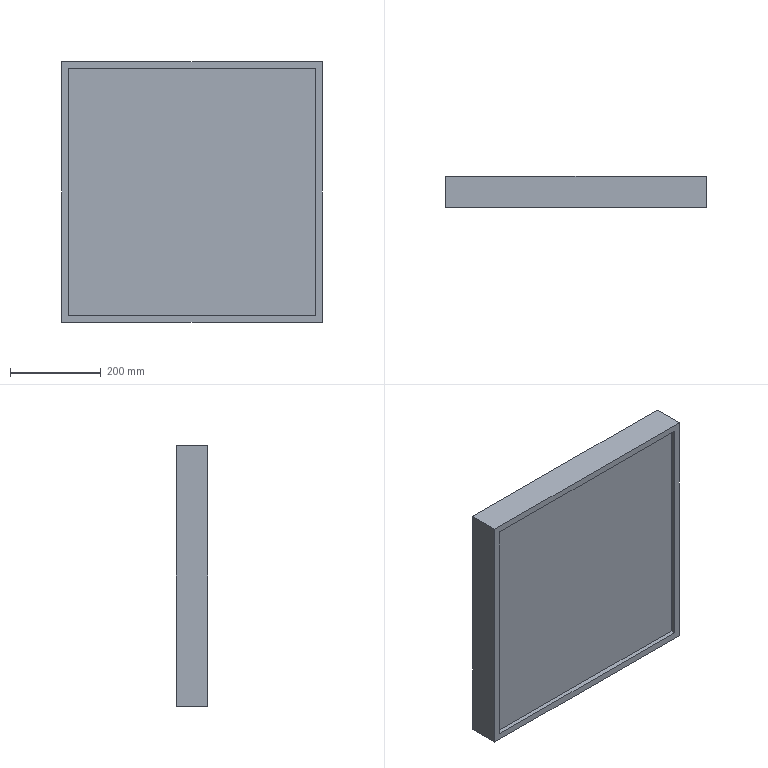Part | STEP file | FFUfilter | 1 solid | 11 faces | box 575 x 69 x 575 mm | volume 19842875 mm3 | plane 11
STEP:
#1=CARTESIAN_POINT('',(0.,0.,0.));
#2=DIRECTION('',(0.,0.,1.));
#3=DIRECTION('',(1.,0.,0.));
#4=AXIS2_PLACEMENT_3D('',#1,#2,#3);
#5=CARTESIAN_POINT('',(-287.5,0.,-287.5));
#6=VERTEX_POINT('',#5);
#7=CARTESIAN_POINT('',(-287.5,0.,287.5));
#8=VERTEX_POINT('',#7);
#9=CARTESIAN_POINT('',(-287.5,0.,-287.5));
#10=DIRECTION('',(0.,0.,1.));
#11=VECTOR('',#10,1.);
#12=LINE('',#9,#11);
#13=CARTESIAN_POINT('',(-287.5,69.,-287.5));
#14=DIRECTION('',(1.,0.,0.));
#15=DIRECTION('',(0.,0.,-1.));
#16=AXIS2_PLACEMENT_3D('',#13,#14,#15);
#17=PLANE('',#16);
#18=CARTESIAN_POINT('',(0.,-69.));
#19=DIRECTION('',(-1.,0.));
#20=VECTOR('',#19,1.);
#21=LINE('',#18,#20);
#22=(GEOMETRIC_REPRESENTATION_CONTEXT(2)PARAMETRIC_REPRESENTATION_CONTEXT()REPRESENTATION_CONTEXT('',''));
#23=DEFINITIONAL_REPRESENTATION('',(#21),#22);
#24=PCURVE('',#17,#23);
#25=CARTESIAN_POINT('',(0.,0.,0.));
#26=DIRECTION('',(0.,1.,0.));
#27=DIRECTION('',(0.,0.,1.));
#28=AXIS2_PLACEMENT_3D('',#25,#26,#27);
#29=PLANE('',#28);
#30=CARTESIAN_POINT('',(-287.5,-287.5));
#31=DIRECTION('',(1.,0.));
#32=VECTOR('',#31,1.);
#33=LINE('',#30,#32);
#34=(GEOMETRIC_REPRESENTATION_CONTEXT(2)PARAMETRIC_REPRESENTATION_CONTEXT()REPRESENTATION_CONTEXT('',''));
#35=DEFINITIONAL_REPRESENTATION('',(#33),#34);
#36=PCURVE('',#29,#35);
#37=SURFACE_CURVE('',#12,(#24,#36),.PCURVE_S1.);
#38=EDGE_CURVE('',#6,#8,#37,.T.);
#39=ORIENTED_EDGE('',*,*,#38,.T.);
#40=CARTESIAN_POINT('',(-287.5,69.,287.5));
#41=VERTEX_POINT('',#40);
#42=CARTESIAN_POINT('',(-287.5,69.,287.5));
#43=DIRECTION('',(0.,-1.,0.));
#44=VECTOR('',#43,1.);
#45=LINE('',#42,#44);
#46=CARTESIAN_POINT('',(-575.,0.));
#47=DIRECTION('',(0.,-1.));
#48=VECTOR('',#47,1.);
#49=LINE('',#46,#48);
#50=(GEOMETRIC_REPRESENTATION_CONTEXT(2)PARAMETRIC_REPRESENTATION_CONTEXT()REPRESENTATION_CONTEXT('',''));
#51=DEFINITIONAL_REPRESENTATION('',(#49),#50);
#52=PCURVE('',#17,#51);
#53=CARTESIAN_POINT('',(-287.5,69.,287.5));
#54=DIRECTION('',(0.,0.,-1.));
#55=DIRECTION('',(-1.,0.,0.));
#56=AXIS2_PLACEMENT_3D('',#53,#54,#55);
#57=PLANE('',#56);
#58=CARTESIAN_POINT('',(0.,0.));
#59=DIRECTION('',(0.,-1.));
#60=VECTOR('',#59,1.);
#61=LINE('',#58,#60);
#62=(GEOMETRIC_REPRESENTATION_CONTEXT(2)PARAMETRIC_REPRESENTATION_CONTEXT()REPRESENTATION_CONTEXT('',''));
#63=DEFINITIONAL_REPRESENTATION('',(#61),#62);
#64=PCURVE('',#57,#63);
#65=SURFACE_CURVE('',#45,(#52,#64),.PCURVE_S1.);
#66=EDGE_CURVE('',#41,#8,#65,.T.);
#67=ORIENTED_EDGE('',*,*,#66,.F.);
#68=CARTESIAN_POINT('',(-287.5,69.,-287.5));
#69=VERTEX_POINT('',#68);
#70=CARTESIAN_POINT('',(-287.5,69.,-287.5));
#71=DIRECTION('',(0.,0.,1.));
#72=VECTOR('',#71,1.);
#73=LINE('',#70,#72);
#74=CARTESIAN_POINT('',(0.,0.));
#75=DIRECTION('',(-1.,0.));
#76=VECTOR('',#75,1.);
#77=LINE('',#74,#76);
#78=(GEOMETRIC_REPRESENTATION_CONTEXT(2)PARAMETRIC_REPRESENTATION_CONTEXT()REPRESENTATION_CONTEXT('',''));
#79=DEFINITIONAL_REPRESENTATION('',(#77),#78);
#80=PCURVE('',#17,#79);
#81=CARTESIAN_POINT('',(0.,69.,0.));
#82=DIRECTION('',(0.,1.,0.));
#83=DIRECTION('',(0.,0.,1.));
#84=AXIS2_PLACEMENT_3D('',#81,#82,#83);
#85=PLANE('',#84);
#86=CARTESIAN_POINT('',(-287.5,-287.5));
#87=DIRECTION('',(1.,0.));
#88=VECTOR('',#87,1.);
#89=LINE('',#86,#88);
#90=(GEOMETRIC_REPRESENTATION_CONTEXT(2)PARAMETRIC_REPRESENTATION_CONTEXT()REPRESENTATION_CONTEXT('',''));
#91=DEFINITIONAL_REPRESENTATION('',(#89),#90);
#92=PCURVE('',#85,#91);
#93=SURFACE_CURVE('',#73,(#80,#92),.PCURVE_S1.);
#94=EDGE_CURVE('',#69,#41,#93,.T.);
#95=ORIENTED_EDGE('',*,*,#94,.F.);
#96=CARTESIAN_POINT('',(-287.5,69.,-287.5));
#97=DIRECTION('',(0.,-1.,0.));
#98=VECTOR('',#97,1.);
#99=LINE('',#96,#98);
#100=CARTESIAN_POINT('',(0.,0.));
#101=DIRECTION('',(0.,-1.));
#102=VECTOR('',#101,1.);
#103=LINE('',#100,#102);
#104=(GEOMETRIC_REPRESENTATION_CONTEXT(2)PARAMETRIC_REPRESENTATION_CONTEXT()REPRESENTATION_CONTEXT('',''));
#105=DEFINITIONAL_REPRESENTATION('',(#103),#104);
#106=PCURVE('',#17,#105);
#107=CARTESIAN_POINT('',(-287.5,69.,-287.5));
#108=DIRECTION('',(0.,0.,1.));
#109=DIRECTION('',(1.,0.,0.));
#110=AXIS2_PLACEMENT_3D('',#107,#108,#109);
#111=PLANE('',#110);
#112=CARTESIAN_POINT('',(0.,0.));
#113=DIRECTION('',(0.,-1.));
#114=VECTOR('',#113,1.);
#115=LINE('',#112,#114);
#116=(GEOMETRIC_REPRESENTATION_CONTEXT(2)PARAMETRIC_REPRESENTATION_CONTEXT()REPRESENTATION_CONTEXT('',''));
#117=DEFINITIONAL_REPRESENTATION('',(#115),#116);
#118=PCURVE('',#111,#117);
#119=SURFACE_CURVE('',#99,(#106,#118),.PCURVE_S1.);
#120=EDGE_CURVE('',#69,#6,#119,.T.);
#121=ORIENTED_EDGE('',*,*,#120,.T.);
#122=EDGE_LOOP('',(#39,#67,#95,#121));
#123=FACE_BOUND('',#122,.T.);
#124=ADVANCED_FACE('',(#123),#17,.F.);
#125=CARTESIAN_POINT('',(287.5,0.,287.5));
#126=VERTEX_POINT('',#125);
#127=CARTESIAN_POINT('',(-287.5,0.,287.5));
#128=DIRECTION('',(1.,0.,0.));
#129=VECTOR('',#128,1.);
#130=LINE('',#127,#129);
#131=CARTESIAN_POINT('',(0.,-69.));
#132=DIRECTION('',(-1.,0.));
#133=VECTOR('',#132,1.);
#134=LINE('',#131,#133);
#135=(GEOMETRIC_REPRESENTATION_CONTEXT(2)PARAMETRIC_REPRESENTATION_CONTEXT()REPRESENTATION_CONTEXT('',''));
#136=DEFINITIONAL_REPRESENTATION('',(#134),#135);
#137=PCURVE('',#57,#136);
#138=CARTESIAN_POINT('',(287.5,-287.5));
#139=DIRECTION('',(0.,1.));
#140=VECTOR('',#139,1.);
#141=LINE('',#138,#140);
#142=(GEOMETRIC_REPRESENTATION_CONTEXT(2)PARAMETRIC_REPRESENTATION_CONTEXT()REPRESENTATION_CONTEXT('',''));
#143=DEFINITIONAL_REPRESENTATION('',(#141),#142);
#144=PCURVE('',#29,#143);
#145=SURFACE_CURVE('',#130,(#137,#144),.PCURVE_S1.);
#146=EDGE_CURVE('',#8,#126,#145,.T.);
#147=ORIENTED_EDGE('',*,*,#146,.T.);
#148=CARTESIAN_POINT('',(287.5,69.,287.5));
#149=VERTEX_POINT('',#148);
#150=CARTESIAN_POINT('',(287.5,69.,287.5));
#151=DIRECTION('',(0.,-1.,0.));
#152=VECTOR('',#151,1.);
#153=LINE('',#150,#152);
#154=CARTESIAN_POINT('',(-575.,0.));
#155=DIRECTION('',(0.,-1.));
#156=VECTOR('',#155,1.);
#157=LINE('',#154,#156);
#158=(GEOMETRIC_REPRESENTATION_CONTEXT(2)PARAMETRIC_REPRESENTATION_CONTEXT()REPRESENTATION_CONTEXT('',''));
#159=DEFINITIONAL_REPRESENTATION('',(#157),#158);
#160=PCURVE('',#57,#159);
#161=CARTESIAN_POINT('',(287.5,69.,-287.5));
#162=DIRECTION('',(-1.,0.,0.));
#163=DIRECTION('',(0.,0.,1.));
#164=AXIS2_PLACEMENT_3D('',#161,#162,#163);
#165=PLANE('',#164);
#166=CARTESIAN_POINT('',(575.,0.));
#167=DIRECTION('',(0.,-1.));
#168=VECTOR('',#167,1.);
#169=LINE('',#166,#168);
#170=(GEOMETRIC_REPRESENTATION_CONTEXT(2)PARAMETRIC_REPRESENTATION_CONTEXT()REPRESENTATION_CONTEXT('',''));
#171=DEFINITIONAL_REPRESENTATION('',(#169),#170);
#172=PCURVE('',#165,#171);
#173=SURFACE_CURVE('',#153,(#160,#172),.PCURVE_S1.);
#174=EDGE_CURVE('',#149,#126,#173,.T.);
#175=ORIENTED_EDGE('',*,*,#174,.F.);
#176=CARTESIAN_POINT('',(-287.5,69.,287.5));
#177=DIRECTION('',(1.,0.,0.));
#178=VECTOR('',#177,1.);
#179=LINE('',#176,#178);
#180=CARTESIAN_POINT('',(0.,0.));
#181=DIRECTION('',(-1.,0.));
#182=VECTOR('',#181,1.);
#183=LINE('',#180,#182);
#184=(GEOMETRIC_REPRESENTATION_CONTEXT(2)PARAMETRIC_REPRESENTATION_CONTEXT()REPRESENTATION_CONTEXT('',''));
#185=DEFINITIONAL_REPRESENTATION('',(#183),#184);
#186=PCURVE('',#57,#185);
#187=CARTESIAN_POINT('',(287.5,-287.5));
#188=DIRECTION('',(0.,1.));
#189=VECTOR('',#188,1.);
#190=LINE('',#187,#189);
#191=(GEOMETRIC_REPRESENTATION_CONTEXT(2)PARAMETRIC_REPRESENTATION_CONTEXT()REPRESENTATION_CONTEXT('',''));
#192=DEFINITIONAL_REPRESENTATION('',(#190),#191);
#193=PCURVE('',#85,#192);
#194=SURFACE_CURVE('',#179,(#186,#193),.PCURVE_S1.);
#195=EDGE_CURVE('',#41,#149,#194,.T.);
#196=ORIENTED_EDGE('',*,*,#195,.F.);
#197=ORIENTED_EDGE('',*,*,#66,.T.);
#198=EDGE_LOOP('',(#147,#175,#196,#197));
#199=FACE_BOUND('',#198,.T.);
#200=ADVANCED_FACE('',(#199),#57,.F.);
#201=CARTESIAN_POINT('',(287.5,0.,-287.5));
#202=VERTEX_POINT('',#201);
#203=CARTESIAN_POINT('',(287.5,0.,-287.5));
#204=DIRECTION('',(0.,0.,-1.));
#205=VECTOR('',#204,1.);
#206=LINE('',#203,#205);
#207=CARTESIAN_POINT('',(0.,-69.));
#208=DIRECTION('',(-1.,0.));
#209=VECTOR('',#208,1.);
#210=LINE('',#207,#209);
#211=(GEOMETRIC_REPRESENTATION_CONTEXT(2)PARAMETRIC_REPRESENTATION_CONTEXT()REPRESENTATION_CONTEXT('',''));
#212=DEFINITIONAL_REPRESENTATION('',(#210),#211);
#213=PCURVE('',#165,#212);
#214=CARTESIAN_POINT('',(-287.5,287.5));
#215=DIRECTION('',(-1.,0.));
#216=VECTOR('',#215,1.);
#217=LINE('',#214,#216);
#218=(GEOMETRIC_REPRESENTATION_CONTEXT(2)PARAMETRIC_REPRESENTATION_CONTEXT()REPRESENTATION_CONTEXT('',''));
#219=DEFINITIONAL_REPRESENTATION('',(#217),#218);
#220=PCURVE('',#29,#219);
#221=SURFACE_CURVE('',#206,(#213,#220),.PCURVE_S1.);
#222=EDGE_CURVE('',#126,#202,#221,.T.);
#223=ORIENTED_EDGE('',*,*,#222,.T.);
#224=CARTESIAN_POINT('',(287.5,69.,-287.5));
#225=VERTEX_POINT('',#224);
#226=CARTESIAN_POINT('',(287.5,69.,-287.5));
#227=DIRECTION('',(0.,-1.,0.));
#228=VECTOR('',#227,1.);
#229=LINE('',#226,#228);
#230=CARTESIAN_POINT('',(0.,0.));
#231=DIRECTION('',(0.,-1.));
#232=VECTOR('',#231,1.);
#233=LINE('',#230,#232);
#234=(GEOMETRIC_REPRESENTATION_CONTEXT(2)PARAMETRIC_REPRESENTATION_CONTEXT()REPRESENTATION_CONTEXT('',''));
#235=DEFINITIONAL_REPRESENTATION('',(#233),#234);
#236=PCURVE('',#165,#235);
#237=CARTESIAN_POINT('',(575.,0.));
#238=DIRECTION('',(0.,-1.));
#239=VECTOR('',#238,1.);
#240=LINE('',#237,#239);
#241=(GEOMETRIC_REPRESENTATION_CONTEXT(2)PARAMETRIC_REPRESENTATION_CONTEXT()REPRESENTATION_CONTEXT('',''));
#242=DEFINITIONAL_REPRESENTATION('',(#240),#241);
#243=PCURVE('',#111,#242);
#244=SURFACE_CURVE('',#229,(#236,#243),.PCURVE_S1.);
#245=EDGE_CURVE('',#225,#202,#244,.T.);
#246=ORIENTED_EDGE('',*,*,#245,.F.);
#247=CARTESIAN_POINT('',(287.5,69.,-287.5));
#248=DIRECTION('',(0.,0.,-1.));
#249=VECTOR('',#248,1.);
#250=LINE('',#247,#249);
#251=CARTESIAN_POINT('',(0.,0.));
#252=DIRECTION('',(-1.,0.));
#253=VECTOR('',#252,1.);
#254=LINE('',#251,#253);
#255=(GEOMETRIC_REPRESENTATION_CONTEXT(2)PARAMETRIC_REPRESENTATION_CONTEXT()REPRESENTATION_CONTEXT('',''));
#256=DEFINITIONAL_REPRESENTATION('',(#254),#255);
#257=PCURVE('',#165,#256);
#258=CARTESIAN_POINT('',(-287.5,287.5));
#259=DIRECTION('',(-1.,0.));
#260=VECTOR('',#259,1.);
#261=LINE('',#258,#260);
#262=(GEOMETRIC_REPRESENTATION_CONTEXT(2)PARAMETRIC_REPRESENTATION_CONTEXT()REPRESENTATION_CONTEXT('',''));
#263=DEFINITIONAL_REPRESENTATION('',(#261),#262);
#264=PCURVE('',#85,#263);
#265=SURFACE_CURVE('',#250,(#257,#264),.PCURVE_S1.);
#266=EDGE_CURVE('',#149,#225,#265,.T.);
#267=ORIENTED_EDGE('',*,*,#266,.F.);
#268=ORIENTED_EDGE('',*,*,#174,.T.);
#269=EDGE_LOOP('',(#223,#246,#267,#268));
#270=FACE_BOUND('',#269,.T.);
#271=ADVANCED_FACE('',(#270),#165,.F.);
#272=CARTESIAN_POINT('',(-287.5,0.,-287.5));
#273=DIRECTION('',(-1.,0.,0.));
#274=VECTOR('',#273,1.);
#275=LINE('',#272,#274);
#276=CARTESIAN_POINT('',(0.,-69.));
#277=DIRECTION('',(-1.,0.));
#278=VECTOR('',#277,1.);
#279=LINE('',#276,#278);
#280=(GEOMETRIC_REPRESENTATION_CONTEXT(2)PARAMETRIC_REPRESENTATION_CONTEXT()REPRESENTATION_CONTEXT('',''));
#281=DEFINITIONAL_REPRESENTATION('',(#279),#280);
#282=PCURVE('',#111,#281);
#283=CARTESIAN_POINT('',(-287.5,-287.5));
#284=DIRECTION('',(0.,-1.));
#285=VECTOR('',#284,1.);
#286=LINE('',#283,#285);
#287=(GEOMETRIC_REPRESENTATION_CONTEXT(2)PARAMETRIC_REPRESENTATION_CONTEXT()REPRESENTATION_CONTEXT('',''));
#288=DEFINITIONAL_REPRESENTATION('',(#286),#287);
#289=PCURVE('',#29,#288);
#290=SURFACE_CURVE('',#275,(#282,#289),.PCURVE_S1.);
#291=EDGE_CURVE('',#202,#6,#290,.T.);
#292=ORIENTED_EDGE('',*,*,#291,.T.);
#293=ORIENTED_EDGE('',*,*,#120,.F.);
#294=CARTESIAN_POINT('',(-287.5,69.,-287.5));
#295=DIRECTION('',(-1.,0.,0.));
#296=VECTOR('',#295,1.);
#297=LINE('',#294,#296);
#298=CARTESIAN_POINT('',(0.,0.));
#299=DIRECTION('',(-1.,0.));
#300=VECTOR('',#299,1.);
#301=LINE('',#298,#300);
#302=(GEOMETRIC_REPRESENTATION_CONTEXT(2)PARAMETRIC_REPRESENTATION_CONTEXT()REPRESENTATION_CONTEXT('',''));
#303=DEFINITIONAL_REPRESENTATION('',(#301),#302);
#304=PCURVE('',#111,#303);
#305=CARTESIAN_POINT('',(-287.5,-287.5));
#306=DIRECTION('',(0.,-1.));
#307=VECTOR('',#306,1.);
#308=LINE('',#305,#307);
#309=(GEOMETRIC_REPRESENTATION_CONTEXT(2)PARAMETRIC_REPRESENTATION_CONTEXT()REPRESENTATION_CONTEXT('',''));
#310=DEFINITIONAL_REPRESENTATION('',(#308),#309);
#311=PCURVE('',#85,#310);
#312=SURFACE_CURVE('',#297,(#304,#311),.PCURVE_S1.);
#313=EDGE_CURVE('',#225,#69,#312,.T.);
#314=ORIENTED_EDGE('',*,*,#313,.F.);
#315=ORIENTED_EDGE('',*,*,#245,.T.);
#316=EDGE_LOOP('',(#292,#293,#314,#315));
#317=FACE_BOUND('',#316,.T.);
#318=ADVANCED_FACE('',(#317),#111,.F.);
#319=ORIENTED_EDGE('',*,*,#94,.T.);
#320=ORIENTED_EDGE('',*,*,#195,.T.);
#321=ORIENTED_EDGE('',*,*,#266,.T.);
#322=ORIENTED_EDGE('',*,*,#313,.T.);
#323=EDGE_LOOP('',(#319,#320,#321,#322));
#324=FACE_BOUND('',#323,.T.);
#325=ADVANCED_FACE('',(#324),#85,.T.);
#326=CARTESIAN_POINT('',(-272.5,0.,-272.5));
#327=VERTEX_POINT('',#326);
#328=CARTESIAN_POINT('',(272.5,0.,-272.5));
#329=VERTEX_POINT('',#328);
#330=CARTESIAN_POINT('',(-272.5,0.,-272.5));
#331=DIRECTION('',(1.,0.,0.));
#332=VECTOR('',#331,1.);
#333=LINE('',#330,#332);
#334=CARTESIAN_POINT('',(-272.5,-272.5));
#335=DIRECTION('',(0.,1.));
#336=VECTOR('',#335,1.);
#337=LINE('',#334,#336);
#338=(GEOMETRIC_REPRESENTATION_CONTEXT(2)PARAMETRIC_REPRESENTATION_CONTEXT()REPRESENTATION_CONTEXT('',''));
#339=DEFINITIONAL_REPRESENTATION('',(#337),#338);
#340=PCURVE('',#29,#339);
#341=CARTESIAN_POINT('',(-272.5,10.,-272.5));
#342=DIRECTION('',(0.,0.,-1.));
#343=DIRECTION('',(-1.,0.,0.));
#344=AXIS2_PLACEMENT_3D('',#341,#342,#343);
#345=PLANE('',#344);
#346=CARTESIAN_POINT('',(0.,-10.));
#347=DIRECTION('',(-1.,0.));
#348=VECTOR('',#347,1.);
#349=LINE('',#346,#348);
#350=(GEOMETRIC_REPRESENTATION_CONTEXT(2)PARAMETRIC_REPRESENTATION_CONTEXT()REPRESENTATION_CONTEXT('',''));
#351=DEFINITIONAL_REPRESENTATION('',(#349),#350);
#352=PCURVE('',#345,#351);
#353=SURFACE_CURVE('',#333,(#340,#352),.PCURVE_S1.);
#354=EDGE_CURVE('',#327,#329,#353,.T.);
#355=ORIENTED_EDGE('',*,*,#354,.F.);
#356=CARTESIAN_POINT('',(-272.5,0.,272.5));
#357=VERTEX_POINT('',#356);
#358=CARTESIAN_POINT('',(-272.5,0.,272.5));
#359=DIRECTION('',(0.,0.,-1.));
#360=VECTOR('',#359,1.);
#361=LINE('',#358,#360);
#362=CARTESIAN_POINT('',(272.5,-272.5));
#363=DIRECTION('',(-1.,0.));
#364=VECTOR('',#363,1.);
#365=LINE('',#362,#364);
#366=(GEOMETRIC_REPRESENTATION_CONTEXT(2)PARAMETRIC_REPRESENTATION_CONTEXT()REPRESENTATION_CONTEXT('',''));
#367=DEFINITIONAL_REPRESENTATION('',(#365),#366);
#368=PCURVE('',#29,#367);
#369=CARTESIAN_POINT('',(-272.5,10.,272.5));
#370=DIRECTION('',(-1.,0.,0.));
#371=DIRECTION('',(0.,0.,1.));
#372=AXIS2_PLACEMENT_3D('',#369,#370,#371);
#373=PLANE('',#372);
#374=CARTESIAN_POINT('',(0.,-10.));
#375=DIRECTION('',(-1.,0.));
#376=VECTOR('',#375,1.);
#377=LINE('',#374,#376);
#378=(GEOMETRIC_REPRESENTATION_CONTEXT(2)PARAMETRIC_REPRESENTATION_CONTEXT()REPRESENTATION_CONTEXT('',''));
#379=DEFINITIONAL_REPRESENTATION('',(#377),#378);
#380=PCURVE('',#373,#379);
#381=SURFACE_CURVE('',#361,(#368,#380),.PCURVE_S1.);
#382=EDGE_CURVE('',#357,#327,#381,.T.);
#383=ORIENTED_EDGE('',*,*,#382,.F.);
#384=CARTESIAN_POINT('',(272.5,0.,272.5));
#385=VERTEX_POINT('',#384);
#386=CARTESIAN_POINT('',(-272.5,0.,272.5));
#387=DIRECTION('',(-1.,0.,0.));
#388=VECTOR('',#387,1.);
#389=LINE('',#386,#388);
#390=CARTESIAN_POINT('',(272.5,-272.5));
#391=DIRECTION('',(0.,-1.));
#392=VECTOR('',#391,1.);
#393=LINE('',#390,#392);
#394=(GEOMETRIC_REPRESENTATION_CONTEXT(2)PARAMETRIC_REPRESENTATION_CONTEXT()REPRESENTATION_CONTEXT('',''));
#395=DEFINITIONAL_REPRESENTATION('',(#393),#394);
#396=PCURVE('',#29,#395);
#397=CARTESIAN_POINT('',(-272.5,10.,272.5));
#398=DIRECTION('',(0.,0.,1.));
#399=DIRECTION('',(1.,0.,0.));
#400=AXIS2_PLACEMENT_3D('',#397,#398,#399);
#401=PLANE('',#400);
#402=CARTESIAN_POINT('',(0.,-10.));
#403=DIRECTION('',(-1.,0.));
#404=VECTOR('',#403,1.);
#405=LINE('',#402,#404);
#406=(GEOMETRIC_REPRESENTATION_CONTEXT(2)PARAMETRIC_REPRESENTATION_CONTEXT()REPRESENTATION_CONTEXT('',''));
#407=DEFINITIONAL_REPRESENTATION('',(#405),#406);
#408=PCURVE('',#401,#407);
#409=SURFACE_CURVE('',#389,(#396,#408),.PCURVE_S1.);
#410=EDGE_CURVE('',#385,#357,#409,.T.);
#411=ORIENTED_EDGE('',*,*,#410,.F.);
#412=CARTESIAN_POINT('',(272.5,0.,272.5));
#413=DIRECTION('',(0.,0.,1.));
#414=VECTOR('',#413,1.);
#415=LINE('',#412,#414);
#416=CARTESIAN_POINT('',(272.5,272.5));
#417=DIRECTION('',(1.,0.));
#418=VECTOR('',#417,1.);
#419=LINE('',#416,#418);
#420=(GEOMETRIC_REPRESENTATION_CONTEXT(2)PARAMETRIC_REPRESENTATION_CONTEXT()REPRESENTATION_CONTEXT('',''));
#421=DEFINITIONAL_REPRESENTATION('',(#419),#420);
#422=PCURVE('',#29,#421);
#423=CARTESIAN_POINT('',(272.5,10.,272.5));
#424=DIRECTION('',(1.,0.,0.));
#425=DIRECTION('',(0.,0.,-1.));
#426=AXIS2_PLACEMENT_3D('',#423,#424,#425);
#427=PLANE('',#426);
#428=CARTESIAN_POINT('',(0.,-10.));
#429=DIRECTION('',(-1.,0.));
#430=VECTOR('',#429,1.);
#431=LINE('',#428,#430);
#432=(GEOMETRIC_REPRESENTATION_CONTEXT(2)PARAMETRIC_REPRESENTATION_CONTEXT()REPRESENTATION_CONTEXT('',''));
#433=DEFINITIONAL_REPRESENTATION('',(#431),#432);
#434=PCURVE('',#427,#433);
#435=SURFACE_CURVE('',#415,(#422,#434),.PCURVE_S1.);
#436=EDGE_CURVE('',#329,#385,#435,.T.);
#437=ORIENTED_EDGE('',*,*,#436,.F.);
#438=EDGE_LOOP('',(#355,#383,#411,#437));
#439=FACE_BOUND('',#438,.T.);
#440=ORIENTED_EDGE('',*,*,#38,.F.);
#441=ORIENTED_EDGE('',*,*,#291,.F.);
#442=ORIENTED_EDGE('',*,*,#222,.F.);
#443=ORIENTED_EDGE('',*,*,#146,.F.);
#444=EDGE_LOOP('',(#440,#441,#442,#443));
#445=FACE_BOUND('',#444,.T.);
#446=ADVANCED_FACE('',(#439,#445),#29,.F.);
#447=ORIENTED_EDGE('',*,*,#382,.T.);
#448=CARTESIAN_POINT('',(-272.5,10.,-272.5));
#449=VERTEX_POINT('',#448);
#450=CARTESIAN_POINT('',(-272.5,10.,-272.5));
#451=DIRECTION('',(0.,-1.,0.));
#452=VECTOR('',#451,1.);
#453=LINE('',#450,#452);
#454=CARTESIAN_POINT('',(-545.,0.));
#455=DIRECTION('',(0.,-1.));
#456=VECTOR('',#455,1.);
#457=LINE('',#454,#456);
#458=(GEOMETRIC_REPRESENTATION_CONTEXT(2)PARAMETRIC_REPRESENTATION_CONTEXT()REPRESENTATION_CONTEXT('',''));
#459=DEFINITIONAL_REPRESENTATION('',(#457),#458);
#460=PCURVE('',#373,#459);
#461=CARTESIAN_POINT('',(0.,0.));
#462=DIRECTION('',(0.,-1.));
#463=VECTOR('',#462,1.);
#464=LINE('',#461,#463);
#465=(GEOMETRIC_REPRESENTATION_CONTEXT(2)PARAMETRIC_REPRESENTATION_CONTEXT()REPRESENTATION_CONTEXT('',''));
#466=DEFINITIONAL_REPRESENTATION('',(#464),#465);
#467=PCURVE('',#345,#466);
#468=SURFACE_CURVE('',#453,(#460,#467),.PCURVE_S1.);
#469=EDGE_CURVE('',#449,#327,#468,.T.);
#470=ORIENTED_EDGE('',*,*,#469,.F.);
#471=CARTESIAN_POINT('',(-272.5,10.,272.5));
#472=VERTEX_POINT('',#471);
#473=CARTESIAN_POINT('',(-272.5,10.,272.5));
#474=DIRECTION('',(0.,0.,-1.));
#475=VECTOR('',#474,1.);
#476=LINE('',#473,#475);
#477=CARTESIAN_POINT('',(0.,0.));
#478=DIRECTION('',(-1.,0.));
#479=VECTOR('',#478,1.);
#480=LINE('',#477,#479);
#481=(GEOMETRIC_REPRESENTATION_CONTEXT(2)PARAMETRIC_REPRESENTATION_CONTEXT()REPRESENTATION_CONTEXT('',''));
#482=DEFINITIONAL_REPRESENTATION('',(#480),#481);
#483=PCURVE('',#373,#482);
#484=CARTESIAN_POINT('',(0.,10.,0.));
#485=DIRECTION('',(0.,-1.,0.));
#486=DIRECTION('',(0.,0.,-1.));
#487=AXIS2_PLACEMENT_3D('',#484,#485,#486);
#488=PLANE('',#487);
#489=CARTESIAN_POINT('',(-272.5,-272.5));
#490=DIRECTION('',(1.,0.));
#491=VECTOR('',#490,1.);
#492=LINE('',#489,#491);
#493=(GEOMETRIC_REPRESENTATION_CONTEXT(2)PARAMETRIC_REPRESENTATION_CONTEXT()REPRESENTATION_CONTEXT('',''));
#494=DEFINITIONAL_REPRESENTATION('',(#492),#493);
#495=PCURVE('',#488,#494);
#496=SURFACE_CURVE('',#476,(#483,#495),.PCURVE_S1.);
#497=EDGE_CURVE('',#472,#449,#496,.T.);
#498=ORIENTED_EDGE('',*,*,#497,.F.);
#499=CARTESIAN_POINT('',(-272.5,10.,272.5));
#500=DIRECTION('',(0.,-1.,0.));
#501=VECTOR('',#500,1.);
#502=LINE('',#499,#501);
#503=CARTESIAN_POINT('',(0.,0.));
#504=DIRECTION('',(0.,-1.));
#505=VECTOR('',#504,1.);
#506=LINE('',#503,#505);
#507=(GEOMETRIC_REPRESENTATION_CONTEXT(2)PARAMETRIC_REPRESENTATION_CONTEXT()REPRESENTATION_CONTEXT('',''));
#508=DEFINITIONAL_REPRESENTATION('',(#506),#507);
#509=PCURVE('',#373,#508);
#510=CARTESIAN_POINT('',(0.,0.));
#511=DIRECTION('',(0.,-1.));
#512=VECTOR('',#511,1.);
#513=LINE('',#510,#512);
#514=(GEOMETRIC_REPRESENTATION_CONTEXT(2)PARAMETRIC_REPRESENTATION_CONTEXT()REPRESENTATION_CONTEXT('',''));
#515=DEFINITIONAL_REPRESENTATION('',(#513),#514);
#516=PCURVE('',#401,#515);
#517=SURFACE_CURVE('',#502,(#509,#516),.PCURVE_S1.);
#518=EDGE_CURVE('',#472,#357,#517,.T.);
#519=ORIENTED_EDGE('',*,*,#518,.T.);
#520=EDGE_LOOP('',(#447,#470,#498,#519));
#521=FACE_BOUND('',#520,.T.);
#522=ADVANCED_FACE('',(#521),#373,.F.);
#523=ORIENTED_EDGE('',*,*,#410,.T.);
#524=ORIENTED_EDGE('',*,*,#518,.F.);
#525=CARTESIAN_POINT('',(272.5,10.,272.5));
#526=VERTEX_POINT('',#525);
#527=CARTESIAN_POINT('',(-272.5,10.,272.5));
#528=DIRECTION('',(-1.,0.,0.));
#529=VECTOR('',#528,1.);
#530=LINE('',#527,#529);
#531=CARTESIAN_POINT('',(0.,0.));
#532=DIRECTION('',(-1.,0.));
#533=VECTOR('',#532,1.);
#534=LINE('',#531,#533);
#535=(GEOMETRIC_REPRESENTATION_CONTEXT(2)PARAMETRIC_REPRESENTATION_CONTEXT()REPRESENTATION_CONTEXT('',''));
#536=DEFINITIONAL_REPRESENTATION('',(#534),#535);
#537=PCURVE('',#401,#536);
#538=CARTESIAN_POINT('',(-272.5,-272.5));
#539=DIRECTION('',(0.,-1.));
#540=VECTOR('',#539,1.);
#541=LINE('',#538,#540);
#542=(GEOMETRIC_REPRESENTATION_CONTEXT(2)PARAMETRIC_REPRESENTATION_CONTEXT()REPRESENTATION_CONTEXT('',''));
#543=DEFINITIONAL_REPRESENTATION('',(#541),#542);
#544=PCURVE('',#488,#543);
#545=SURFACE_CURVE('',#530,(#537,#544),.PCURVE_S1.);
#546=EDGE_CURVE('',#526,#472,#545,.T.);
#547=ORIENTED_EDGE('',*,*,#546,.F.);
#548=CARTESIAN_POINT('',(272.5,10.,272.5));
#549=DIRECTION('',(0.,-1.,0.));
#550=VECTOR('',#549,1.);
#551=LINE('',#548,#550);
#552=CARTESIAN_POINT('',(545.,0.));
#553=DIRECTION('',(0.,-1.));
#554=VECTOR('',#553,1.);
#555=LINE('',#552,#554);
#556=(GEOMETRIC_REPRESENTATION_CONTEXT(2)PARAMETRIC_REPRESENTATION_CONTEXT()REPRESENTATION_CONTEXT('',''));
#557=DEFINITIONAL_REPRESENTATION('',(#555),#556);
#558=PCURVE('',#401,#557);
#559=CARTESIAN_POINT('',(0.,0.));
#560=DIRECTION('',(0.,-1.));
#561=VECTOR('',#560,1.);
#562=LINE('',#559,#561);
#563=(GEOMETRIC_REPRESENTATION_CONTEXT(2)PARAMETRIC_REPRESENTATION_CONTEXT()REPRESENTATION_CONTEXT('',''));
#564=DEFINITIONAL_REPRESENTATION('',(#562),#563);
#565=PCURVE('',#427,#564);
#566=SURFACE_CURVE('',#551,(#558,#565),.PCURVE_S1.);
#567=EDGE_CURVE('',#526,#385,#566,.T.);
#568=ORIENTED_EDGE('',*,*,#567,.T.);
#569=EDGE_LOOP('',(#523,#524,#547,#568));
#570=FACE_BOUND('',#569,.T.);
#571=ADVANCED_FACE('',(#570),#401,.F.);
#572=ORIENTED_EDGE('',*,*,#436,.T.);
#573=ORIENTED_EDGE('',*,*,#567,.F.);
#574=CARTESIAN_POINT('',(272.5,10.,-272.5));
#575=VERTEX_POINT('',#574);
#576=CARTESIAN_POINT('',(272.5,10.,272.5));
#577=DIRECTION('',(0.,0.,1.));
#578=VECTOR('',#577,1.);
#579=LINE('',#576,#578);
#580=CARTESIAN_POINT('',(0.,0.));
#581=DIRECTION('',(-1.,0.));
#582=VECTOR('',#581,1.);
#583=LINE('',#580,#582);
#584=(GEOMETRIC_REPRESENTATION_CONTEXT(2)PARAMETRIC_REPRESENTATION_CONTEXT()REPRESENTATION_CONTEXT('',''));
#585=DEFINITIONAL_REPRESENTATION('',(#583),#584);
#586=PCURVE('',#427,#585);
#587=CARTESIAN_POINT('',(-272.5,272.5));
#588=DIRECTION('',(-1.,0.));
#589=VECTOR('',#588,1.);
#590=LINE('',#587,#589);
#591=(GEOMETRIC_REPRESENTATION_CONTEXT(2)PARAMETRIC_REPRESENTATION_CONTEXT()REPRESENTATION_CONTEXT('',''));
#592=DEFINITIONAL_REPRESENTATION('',(#590),#591);
#593=PCURVE('',#488,#592);
#594=SURFACE_CURVE('',#579,(#586,#593),.PCURVE_S1.);
#595=EDGE_CURVE('',#575,#526,#594,.T.);
#596=ORIENTED_EDGE('',*,*,#595,.F.);
#597=CARTESIAN_POINT('',(272.5,10.,-272.5));
#598=DIRECTION('',(0.,-1.,0.));
#599=VECTOR('',#598,1.);
#600=LINE('',#597,#599);
#601=CARTESIAN_POINT('',(545.,0.));
#602=DIRECTION('',(0.,-1.));
#603=VECTOR('',#602,1.);
#604=LINE('',#601,#603);
#605=(GEOMETRIC_REPRESENTATION_CONTEXT(2)PARAMETRIC_REPRESENTATION_CONTEXT()REPRESENTATION_CONTEXT('',''));
#606=DEFINITIONAL_REPRESENTATION('',(#604),#605);
#607=PCURVE('',#427,#606);
#608=CARTESIAN_POINT('',(-545.,0.));
#609=DIRECTION('',(0.,-1.));
#610=VECTOR('',#609,1.);
#611=LINE('',#608,#610);
#612=(GEOMETRIC_REPRESENTATION_CONTEXT(2)PARAMETRIC_REPRESENTATION_CONTEXT()REPRESENTATION_CONTEXT('',''));
#613=DEFINITIONAL_REPRESENTATION('',(#611),#612);
#614=PCURVE('',#345,#613);
#615=SURFACE_CURVE('',#600,(#607,#614),.PCURVE_S1.);
#616=EDGE_CURVE('',#575,#329,#615,.T.);
#617=ORIENTED_EDGE('',*,*,#616,.T.);
#618=EDGE_LOOP('',(#572,#573,#596,#617));
#619=FACE_BOUND('',#618,.T.);
#620=ADVANCED_FACE('',(#619),#427,.F.);
#621=ORIENTED_EDGE('',*,*,#354,.T.);
#622=ORIENTED_EDGE('',*,*,#616,.F.);
#623=CARTESIAN_POINT('',(-272.5,10.,-272.5));
#624=DIRECTION('',(1.,0.,0.));
#625=VECTOR('',#624,1.);
#626=LINE('',#623,#625);
#627=CARTESIAN_POINT('',(0.,0.));
#628=DIRECTION('',(-1.,0.));
#629=VECTOR('',#628,1.);
#630=LINE('',#627,#629);
#631=(GEOMETRIC_REPRESENTATION_CONTEXT(2)PARAMETRIC_REPRESENTATION_CONTEXT()REPRESENTATION_CONTEXT('',''));
#632=DEFINITIONAL_REPRESENTATION('',(#630),#631);
#633=PCURVE('',#345,#632);
#634=CARTESIAN_POINT('',(272.5,-272.5));
#635=DIRECTION('',(0.,1.));
#636=VECTOR('',#635,1.);
#637=LINE('',#634,#636);
#638=(GEOMETRIC_REPRESENTATION_CONTEXT(2)PARAMETRIC_REPRESENTATION_CONTEXT()REPRESENTATION_CONTEXT('',''));
#639=DEFINITIONAL_REPRESENTATION('',(#637),#638);
#640=PCURVE('',#488,#639);
#641=SURFACE_CURVE('',#626,(#633,#640),.PCURVE_S1.);
#642=EDGE_CURVE('',#449,#575,#641,.T.);
#643=ORIENTED_EDGE('',*,*,#642,.F.);
#644=ORIENTED_EDGE('',*,*,#469,.T.);
#645=EDGE_LOOP('',(#621,#622,#643,#644));
#646=FACE_BOUND('',#645,.T.);
#647=ADVANCED_FACE('',(#646),#345,.F.);
#648=ORIENTED_EDGE('',*,*,#497,.T.);
#649=ORIENTED_EDGE('',*,*,#642,.T.);
#650=ORIENTED_EDGE('',*,*,#595,.T.);
#651=ORIENTED_EDGE('',*,*,#546,.T.);
#652=EDGE_LOOP('',(#648,#649,#650,#651));
#653=FACE_BOUND('',#652,.T.);
#654=ADVANCED_FACE('',(#653),#488,.T.);
#655=CLOSED_SHELL('',(#124,#200,#271,#318,#325,#446,#522,#571,#620,#647,#654));
#656=MANIFOLD_SOLID_BREP('',#655);
#657=(LENGTH_UNIT()NAMED_UNIT(*)SI_UNIT(.MILLI.,.METRE.));
#658=UNCERTAINTY_MEASURE_WITH_UNIT(LENGTH_MEASURE(0.0000001),#657,'','');
#659=(NAMED_UNIT(*)PLANE_ANGLE_UNIT()SI_UNIT($,.RADIAN.));
#660=(NAMED_UNIT(*)SI_UNIT($,.STERADIAN.)SOLID_ANGLE_UNIT());
#661=(GEOMETRIC_REPRESENTATION_CONTEXT(3)GLOBAL_UNCERTAINTY_ASSIGNED_CONTEXT((#658))GLOBAL_UNIT_ASSIGNED_CONTEXT((#657,#659,#660))REPRESENTATION_CONTEXT('',''));
#662=ADVANCED_BREP_SHAPE_REPRESENTATION('',(#4,#656),#661);